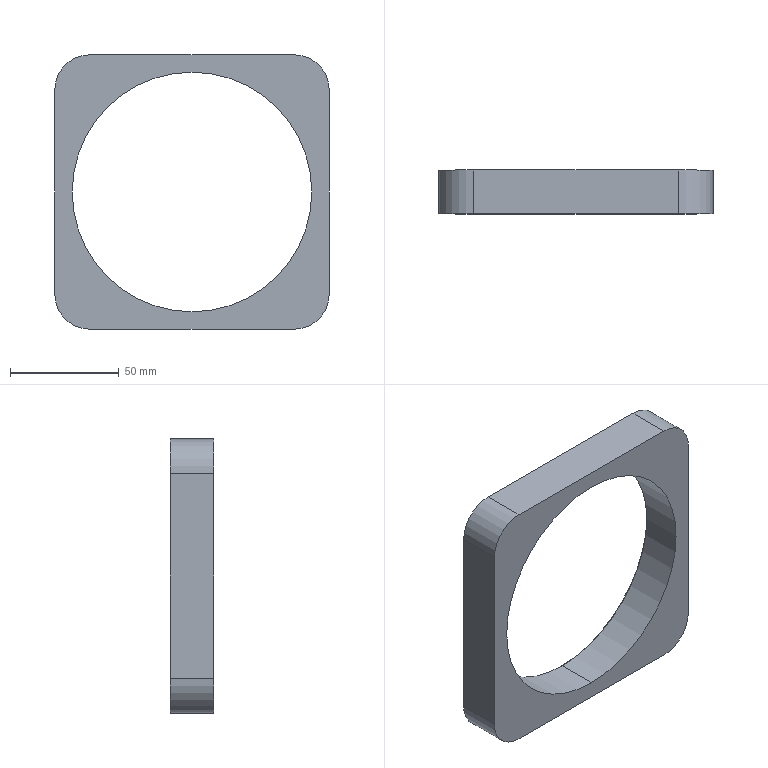Part | SolidWorks | features Chamfer 1, Extrusion 1, HoleWzd 1, ICE 1 | 1 solid | 30 faces | box 126 x 20 x 126 mm | volume 119235 mm3 | cylinder 14 | cone 10 | plane 6 | commonest cylinder face diameters 8.5 x8 32 x4 110 x2
STEP:
#1=CARTESIAN_POINT('',(0.,19.,-55.));
#2=VERTEX_POINT('',#1);
#3=CARTESIAN_POINT('',(0.,19.,55.));
#4=VERTEX_POINT('',#3);
#5=CARTESIAN_POINT('',(0.,19.,0.));
#6=DIRECTION('',(0.,1.,0.));
#7=DIRECTION('',(0.,0.,1.));
#8=AXIS2_PLACEMENT_3D('',#5,#6,#7);
#9=CIRCLE('',#8,55.);
#10=EDGE_CURVE('',#2,#4,#9,.T.);
#11=ORIENTED_EDGE('',*,*,#10,.F.);
#12=CARTESIAN_POINT('',(0.,20.,-56.));
#13=VERTEX_POINT('',#12);
#14=CARTESIAN_POINT('',(0.,19.,-55.));
#15=DIRECTION('',(0.,0.7071,-0.7071));
#16=VECTOR('',#15,1000.);
#17=LINE('',#14,#16);
#18=EDGE_CURVE('',#2,#13,#17,.T.);
#19=ORIENTED_EDGE('',*,*,#18,.T.);
#20=CARTESIAN_POINT('',(0.,20.,56.));
#21=VERTEX_POINT('',#20);
#22=CARTESIAN_POINT('',(0.,20.,0.));
#23=DIRECTION('',(0.,-1.,0.));
#24=DIRECTION('',(0.,0.,1.));
#25=AXIS2_PLACEMENT_3D('',#22,#23,#24);
#26=CIRCLE('',#25,56.);
#27=EDGE_CURVE('',#21,#13,#26,.T.);
#28=ORIENTED_EDGE('',*,*,#27,.F.);
#29=CARTESIAN_POINT('',(0.,19.,55.));
#30=DIRECTION('',(0.,0.7071,0.7071));
#31=VECTOR('',#30,1000.);
#32=LINE('',#29,#31);
#33=EDGE_CURVE('',#4,#21,#32,.T.);
#34=ORIENTED_EDGE('',*,*,#33,.F.);
#35=EDGE_LOOP('',(#11,#19,#28,#34));
#36=FACE_OUTER_BOUND('',#35,.T.);
#37=CARTESIAN_POINT('',(0.,19.,0.));
#38=DIRECTION('',(0.,1.,0.));
#39=DIRECTION('',(0.,0.,1.));
#40=AXIS2_PLACEMENT_3D('',#37,#38,#39);
#41=CONICAL_SURFACE('',#40,55.,0.7854);
#42=ADVANCED_FACE('',(#36),#41,.F.);
#43=CARTESIAN_POINT('',(-47.,4.77,-51.25));
#44=VERTEX_POINT('',#43);
#45=CARTESIAN_POINT('',(-47.,4.77,-42.75));
#46=VERTEX_POINT('',#45);
#47=CARTESIAN_POINT('',(-47.,4.77,-47.));
#48=DIRECTION('',(0.,1.,0.));
#49=DIRECTION('',(0.,0.,1.));
#50=AXIS2_PLACEMENT_3D('',#47,#48,#49);
#51=CIRCLE('',#50,4.25);
#52=EDGE_CURVE('',#44,#46,#51,.T.);
#53=ORIENTED_EDGE('',*,*,#52,.F.);
#54=CARTESIAN_POINT('',(-47.,20.,-51.25));
#55=VERTEX_POINT('',#54);
#56=CARTESIAN_POINT('',(-47.,20.,-51.25));
#57=DIRECTION('',(0.,1.,0.));
#58=VECTOR('',#57,1000.);
#59=LINE('',#56,#58);
#60=EDGE_CURVE('',#44,#55,#59,.T.);
#61=ORIENTED_EDGE('',*,*,#60,.T.);
#62=CARTESIAN_POINT('',(-47.,20.,-42.75));
#63=VERTEX_POINT('',#62);
#64=CARTESIAN_POINT('',(-47.,20.,-47.));
#65=DIRECTION('',(0.,1.,0.));
#66=DIRECTION('',(0.,0.,1.));
#67=AXIS2_PLACEMENT_3D('',#64,#65,#66);
#68=CIRCLE('',#67,4.25);
#69=EDGE_CURVE('',#55,#63,#68,.T.);
#70=ORIENTED_EDGE('',*,*,#69,.T.);
#71=CARTESIAN_POINT('',(-47.,20.,-42.75));
#72=DIRECTION('',(0.,1.,0.));
#73=VECTOR('',#72,1000.);
#74=LINE('',#71,#73);
#75=EDGE_CURVE('',#46,#63,#74,.T.);
#76=ORIENTED_EDGE('',*,*,#75,.F.);
#77=EDGE_LOOP('',(#53,#61,#70,#76));
#78=FACE_OUTER_BOUND('',#77,.T.);
#79=CARTESIAN_POINT('',(-47.,20.,-47.));
#80=DIRECTION('',(0.,1.,0.));
#81=DIRECTION('',(0.,0.,1.));
#82=AXIS2_PLACEMENT_3D('',#79,#80,#81);
#83=CYLINDRICAL_SURFACE('',#82,4.25);
#84=ADVANCED_FACE('',(#78),#83,.F.);
#85=CARTESIAN_POINT('',(-47.,2.216,-47.));
#86=VERTEX_POINT('',#85);
#87=CARTESIAN_POINT('',(-47.,4.77,-42.75));
#88=DIRECTION('',(0.,0.515,0.8572));
#89=VECTOR('',#88,1000.);
#90=LINE('',#87,#89);
#91=EDGE_CURVE('',#86,#46,#90,.T.);
#92=ORIENTED_EDGE('',*,*,#91,.F.);
#93=CARTESIAN_POINT('',(-47.,4.77,-51.25));
#94=DIRECTION('',(0.,0.515,-0.8572));
#95=VECTOR('',#94,1000.);
#96=LINE('',#93,#95);
#97=EDGE_CURVE('',#86,#44,#96,.T.);
#98=ORIENTED_EDGE('',*,*,#97,.T.);
#99=ORIENTED_EDGE('',*,*,#52,.T.);
#100=EDGE_LOOP('',(#92,#98,#99));
#101=FACE_OUTER_BOUND('',#100,.T.);
#102=CARTESIAN_POINT('',(-47.,4.77,-47.));
#103=DIRECTION('',(0.,1.,0.));
#104=DIRECTION('',(0.,0.,1.));
#105=AXIS2_PLACEMENT_3D('',#102,#103,#104);
#106=CONICAL_SURFACE('',#105,4.25,1.03);
#107=ADVANCED_FACE('',(#101),#106,.F.);
#108=CARTESIAN_POINT('',(47.,4.77,-51.25));
#109=VERTEX_POINT('',#108);
#110=CARTESIAN_POINT('',(47.,4.77,-42.75));
#111=VERTEX_POINT('',#110);
#112=CARTESIAN_POINT('',(47.,4.77,-47.));
#113=DIRECTION('',(0.,1.,0.));
#114=DIRECTION('',(0.,0.,1.));
#115=AXIS2_PLACEMENT_3D('',#112,#113,#114);
#116=CIRCLE('',#115,4.25);
#117=EDGE_CURVE('',#109,#111,#116,.T.);
#118=ORIENTED_EDGE('',*,*,#117,.F.);
#119=CARTESIAN_POINT('',(47.,20.,-51.25));
#120=VERTEX_POINT('',#119);
#121=CARTESIAN_POINT('',(47.,20.,-51.25));
#122=DIRECTION('',(0.,1.,0.));
#123=VECTOR('',#122,1000.);
#124=LINE('',#121,#123);
#125=EDGE_CURVE('',#109,#120,#124,.T.);
#126=ORIENTED_EDGE('',*,*,#125,.T.);
#127=CARTESIAN_POINT('',(47.,20.,-42.75));
#128=VERTEX_POINT('',#127);
#129=CARTESIAN_POINT('',(47.,20.,-47.));
#130=DIRECTION('',(0.,1.,0.));
#131=DIRECTION('',(0.,0.,1.));
#132=AXIS2_PLACEMENT_3D('',#129,#130,#131);
#133=CIRCLE('',#132,4.25);
#134=EDGE_CURVE('',#120,#128,#133,.T.);
#135=ORIENTED_EDGE('',*,*,#134,.T.);
#136=CARTESIAN_POINT('',(47.,20.,-42.75));
#137=DIRECTION('',(0.,1.,0.));
#138=VECTOR('',#137,1000.);
#139=LINE('',#136,#138);
#140=EDGE_CURVE('',#111,#128,#139,.T.);
#141=ORIENTED_EDGE('',*,*,#140,.F.);
#142=EDGE_LOOP('',(#118,#126,#135,#141));
#143=FACE_OUTER_BOUND('',#142,.T.);
#144=CARTESIAN_POINT('',(47.,20.,-47.));
#145=DIRECTION('',(0.,1.,0.));
#146=DIRECTION('',(0.,0.,1.));
#147=AXIS2_PLACEMENT_3D('',#144,#145,#146);
#148=CYLINDRICAL_SURFACE('',#147,4.25);
#149=ADVANCED_FACE('',(#143),#148,.F.);
#150=CARTESIAN_POINT('',(47.,2.216,-47.));
#151=VERTEX_POINT('',#150);
#152=CARTESIAN_POINT('',(47.,4.77,-42.75));
#153=DIRECTION('',(0.,0.515,0.8572));
#154=VECTOR('',#153,1000.);
#155=LINE('',#152,#154);
#156=EDGE_CURVE('',#151,#111,#155,.T.);
#157=ORIENTED_EDGE('',*,*,#156,.F.);
#158=CARTESIAN_POINT('',(47.,4.77,-51.25));
#159=DIRECTION('',(0.,0.515,-0.8572));
#160=VECTOR('',#159,1000.);
#161=LINE('',#158,#160);
#162=EDGE_CURVE('',#151,#109,#161,.T.);
#163=ORIENTED_EDGE('',*,*,#162,.T.);
#164=ORIENTED_EDGE('',*,*,#117,.T.);
#165=EDGE_LOOP('',(#157,#163,#164));
#166=FACE_OUTER_BOUND('',#165,.T.);
#167=CARTESIAN_POINT('',(47.,4.77,-47.));
#168=DIRECTION('',(0.,1.,0.));
#169=DIRECTION('',(0.,0.,1.));
#170=AXIS2_PLACEMENT_3D('',#167,#168,#169);
#171=CONICAL_SURFACE('',#170,4.25,1.03);
#172=ADVANCED_FACE('',(#166),#171,.F.);
#173=CARTESIAN_POINT('',(47.,4.77,42.75));
#174=VERTEX_POINT('',#173);
#175=CARTESIAN_POINT('',(47.,4.77,51.25));
#176=VERTEX_POINT('',#175);
#177=CARTESIAN_POINT('',(47.,4.77,47.));
#178=DIRECTION('',(0.,1.,0.));
#179=DIRECTION('',(0.,0.,1.));
#180=AXIS2_PLACEMENT_3D('',#177,#178,#179);
#181=CIRCLE('',#180,4.25);
#182=EDGE_CURVE('',#174,#176,#181,.T.);
#183=ORIENTED_EDGE('',*,*,#182,.F.);
#184=CARTESIAN_POINT('',(47.,20.,42.75));
#185=VERTEX_POINT('',#184);
#186=CARTESIAN_POINT('',(47.,20.,42.75));
#187=DIRECTION('',(0.,1.,0.));
#188=VECTOR('',#187,1000.);
#189=LINE('',#186,#188);
#190=EDGE_CURVE('',#174,#185,#189,.T.);
#191=ORIENTED_EDGE('',*,*,#190,.T.);
#192=CARTESIAN_POINT('',(47.,20.,51.25));
#193=VERTEX_POINT('',#192);
#194=CARTESIAN_POINT('',(47.,20.,47.));
#195=DIRECTION('',(0.,1.,0.));
#196=DIRECTION('',(0.,0.,1.));
#197=AXIS2_PLACEMENT_3D('',#194,#195,#196);
#198=CIRCLE('',#197,4.25);
#199=EDGE_CURVE('',#185,#193,#198,.T.);
#200=ORIENTED_EDGE('',*,*,#199,.T.);
#201=CARTESIAN_POINT('',(47.,20.,51.25));
#202=DIRECTION('',(0.,1.,0.));
#203=VECTOR('',#202,1000.);
#204=LINE('',#201,#203);
#205=EDGE_CURVE('',#176,#193,#204,.T.);
#206=ORIENTED_EDGE('',*,*,#205,.F.);
#207=EDGE_LOOP('',(#183,#191,#200,#206));
#208=FACE_OUTER_BOUND('',#207,.T.);
#209=CARTESIAN_POINT('',(47.,20.,47.));
#210=DIRECTION('',(0.,1.,0.));
#211=DIRECTION('',(0.,0.,1.));
#212=AXIS2_PLACEMENT_3D('',#209,#210,#211);
#213=CYLINDRICAL_SURFACE('',#212,4.25);
#214=ADVANCED_FACE('',(#208),#213,.F.);
#215=CARTESIAN_POINT('',(47.,2.216,47.));
#216=VERTEX_POINT('',#215);
#217=CARTESIAN_POINT('',(47.,4.77,51.25));
#218=DIRECTION('',(0.,0.515,0.8572));
#219=VECTOR('',#218,1000.);
#220=LINE('',#217,#219);
#221=EDGE_CURVE('',#216,#176,#220,.T.);
#222=ORIENTED_EDGE('',*,*,#221,.F.);
#223=CARTESIAN_POINT('',(47.,4.77,42.75));
#224=DIRECTION('',(0.,0.515,-0.8572));
#225=VECTOR('',#224,1000.);
#226=LINE('',#223,#225);
#227=EDGE_CURVE('',#216,#174,#226,.T.);
#228=ORIENTED_EDGE('',*,*,#227,.T.);
#229=ORIENTED_EDGE('',*,*,#182,.T.);
#230=EDGE_LOOP('',(#222,#228,#229));
#231=FACE_OUTER_BOUND('',#230,.T.);
#232=CARTESIAN_POINT('',(47.,4.77,47.));
#233=DIRECTION('',(0.,1.,0.));
#234=DIRECTION('',(0.,0.,1.));
#235=AXIS2_PLACEMENT_3D('',#232,#233,#234);
#236=CONICAL_SURFACE('',#235,4.25,1.03);
#237=ADVANCED_FACE('',(#231),#236,.F.);
#238=CARTESIAN_POINT('',(-47.,4.77,42.75));
#239=VERTEX_POINT('',#238);
#240=CARTESIAN_POINT('',(-47.,4.77,51.25));
#241=VERTEX_POINT('',#240);
#242=CARTESIAN_POINT('',(-47.,4.77,47.));
#243=DIRECTION('',(0.,1.,0.));
#244=DIRECTION('',(0.,0.,1.));
#245=AXIS2_PLACEMENT_3D('',#242,#243,#244);
#246=CIRCLE('',#245,4.25);
#247=EDGE_CURVE('',#239,#241,#246,.T.);
#248=ORIENTED_EDGE('',*,*,#247,.F.);
#249=CARTESIAN_POINT('',(-47.,20.,42.75));
#250=VERTEX_POINT('',#249);
#251=CARTESIAN_POINT('',(-47.,20.,42.75));
#252=DIRECTION('',(0.,1.,0.));
#253=VECTOR('',#252,1000.);
#254=LINE('',#251,#253);
#255=EDGE_CURVE('',#239,#250,#254,.T.);
#256=ORIENTED_EDGE('',*,*,#255,.T.);
#257=CARTESIAN_POINT('',(-47.,20.,51.25));
#258=VERTEX_POINT('',#257);
#259=CARTESIAN_POINT('',(-47.,20.,47.));
#260=DIRECTION('',(0.,1.,0.));
#261=DIRECTION('',(0.,0.,1.));
#262=AXIS2_PLACEMENT_3D('',#259,#260,#261);
#263=CIRCLE('',#262,4.25);
#264=EDGE_CURVE('',#250,#258,#263,.T.);
#265=ORIENTED_EDGE('',*,*,#264,.T.);
#266=CARTESIAN_POINT('',(-47.,20.,51.25));
#267=DIRECTION('',(0.,1.,0.));
#268=VECTOR('',#267,1000.);
#269=LINE('',#266,#268);
#270=EDGE_CURVE('',#241,#258,#269,.T.);
#271=ORIENTED_EDGE('',*,*,#270,.F.);
#272=EDGE_LOOP('',(#248,#256,#265,#271));
#273=FACE_OUTER_BOUND('',#272,.T.);
#274=CARTESIAN_POINT('',(-47.,20.,47.));
#275=DIRECTION('',(0.,1.,0.));
#276=DIRECTION('',(0.,0.,1.));
#277=AXIS2_PLACEMENT_3D('',#274,#275,#276);
#278=CYLINDRICAL_SURFACE('',#277,4.25);
#279=ADVANCED_FACE('',(#273),#278,.F.);
#280=CARTESIAN_POINT('',(-47.,2.216,47.));
#281=VERTEX_POINT('',#280);
#282=CARTESIAN_POINT('',(-47.,4.77,51.25));
#283=DIRECTION('',(0.,0.515,0.8572));
#284=VECTOR('',#283,1000.);
#285=LINE('',#282,#284);
#286=EDGE_CURVE('',#281,#241,#285,.T.);
#287=ORIENTED_EDGE('',*,*,#286,.F.);
#288=CARTESIAN_POINT('',(-47.,4.77,42.75));
#289=DIRECTION('',(0.,0.515,-0.8572));
#290=VECTOR('',#289,1000.);
#291=LINE('',#288,#290);
#292=EDGE_CURVE('',#281,#239,#291,.T.);
#293=ORIENTED_EDGE('',*,*,#292,.T.);
#294=ORIENTED_EDGE('',*,*,#247,.T.);
#295=EDGE_LOOP('',(#287,#293,#294));
#296=FACE_OUTER_BOUND('',#295,.T.);
#297=CARTESIAN_POINT('',(-47.,4.77,47.));
#298=DIRECTION('',(0.,1.,0.));
#299=DIRECTION('',(0.,0.,1.));
#300=AXIS2_PLACEMENT_3D('',#297,#298,#299);
#301=CONICAL_SURFACE('',#300,4.25,1.03);
#302=ADVANCED_FACE('',(#296),#301,.F.);
#303=ORIENTED_EDGE('',*,*,#10,.T.);
#304=CARTESIAN_POINT('',(0.,0.,55.));
#305=VERTEX_POINT('',#304);
#306=CARTESIAN_POINT('',(0.,20.,55.));
#307=DIRECTION('',(0.,-1.,0.));
#308=VECTOR('',#307,1000.);
#309=LINE('',#306,#308);
#310=EDGE_CURVE('',#4,#305,#309,.T.);
#311=ORIENTED_EDGE('',*,*,#310,.T.);
#312=CARTESIAN_POINT('',(0.,0.,-55.));
#313=VERTEX_POINT('',#312);
#314=CARTESIAN_POINT('',(0.,0.,0.));
#315=DIRECTION('',(0.,1.,0.));
#316=DIRECTION('',(0.,0.,1.));
#317=AXIS2_PLACEMENT_3D('',#314,#315,#316);
#318=CIRCLE('',#317,55.);
#319=EDGE_CURVE('',#313,#305,#318,.T.);
#320=ORIENTED_EDGE('',*,*,#319,.F.);
#321=CARTESIAN_POINT('',(0.,20.,-55.));
#322=DIRECTION('',(0.,-1.,0.));
#323=VECTOR('',#322,1000.);
#324=LINE('',#321,#323);
#325=EDGE_CURVE('',#2,#313,#324,.T.);
#326=ORIENTED_EDGE('',*,*,#325,.F.);
#327=EDGE_LOOP('',(#303,#311,#320,#326));
#328=FACE_OUTER_BOUND('',#327,.T.);
#329=CARTESIAN_POINT('',(0.,20.,0.));
#330=DIRECTION('',(0.,-1.,0.));
#331=DIRECTION('',(0.,0.,-1.));
#332=AXIS2_PLACEMENT_3D('',#329,#330,#331);
#333=CYLINDRICAL_SURFACE('',#332,55.);
#334=ADVANCED_FACE('',(#328),#333,.F.);
#335=ORIENTED_EDGE('',*,*,#27,.T.);
#336=CARTESIAN_POINT('',(0.,20.,0.));
#337=DIRECTION('',(0.,-1.,0.));
#338=DIRECTION('',(0.,0.,1.));
#339=AXIS2_PLACEMENT_3D('',#336,#337,#338);
#340=CIRCLE('',#339,56.);
#341=EDGE_CURVE('',#13,#21,#340,.T.);
#342=ORIENTED_EDGE('',*,*,#341,.T.);
#343=EDGE_LOOP('',(#335,#342));
#344=FACE_BOUND('',#343,.T.);
#345=CARTESIAN_POINT('',(-47.,20.,-47.));
#346=DIRECTION('',(0.,1.,0.));
#347=DIRECTION('',(0.,0.,1.));
#348=AXIS2_PLACEMENT_3D('',#345,#346,#347);
#349=CIRCLE('',#348,4.25);
#350=EDGE_CURVE('',#63,#55,#349,.T.);
#351=ORIENTED_EDGE('',*,*,#350,.F.);
#352=ORIENTED_EDGE('',*,*,#69,.F.);
#353=EDGE_LOOP('',(#351,#352));
#354=FACE_BOUND('',#353,.T.);
#355=CARTESIAN_POINT('',(47.,20.,-47.));
#356=DIRECTION('',(0.,1.,0.));
#357=DIRECTION('',(0.,0.,1.));
#358=AXIS2_PLACEMENT_3D('',#355,#356,#357);
#359=CIRCLE('',#358,4.25);
#360=EDGE_CURVE('',#128,#120,#359,.T.);
#361=ORIENTED_EDGE('',*,*,#360,.F.);
#362=ORIENTED_EDGE('',*,*,#134,.F.);
#363=EDGE_LOOP('',(#361,#362));
#364=FACE_BOUND('',#363,.T.);
#365=CARTESIAN_POINT('',(47.,20.,47.));
#366=DIRECTION('',(0.,1.,0.));
#367=DIRECTION('',(0.,0.,1.));
#368=AXIS2_PLACEMENT_3D('',#365,#366,#367);
#369=CIRCLE('',#368,4.25);
#370=EDGE_CURVE('',#193,#185,#369,.T.);
#371=ORIENTED_EDGE('',*,*,#370,.F.);
#372=ORIENTED_EDGE('',*,*,#199,.F.);
#373=EDGE_LOOP('',(#371,#372));
#374=FACE_BOUND('',#373,.T.);
#375=CARTESIAN_POINT('',(-47.,20.,47.));
#376=DIRECTION('',(0.,1.,0.));
#377=DIRECTION('',(0.,0.,1.));
#378=AXIS2_PLACEMENT_3D('',#375,#376,#377);
#379=CIRCLE('',#378,4.25);
#380=EDGE_CURVE('',#258,#250,#379,.T.);
#381=ORIENTED_EDGE('',*,*,#380,.F.);
#382=ORIENTED_EDGE('',*,*,#264,.F.);
#383=EDGE_LOOP('',(#381,#382));
#384=FACE_BOUND('',#383,.T.);
#385=CARTESIAN_POINT('',(-63.,20.,47.));
#386=VERTEX_POINT('',#385);
#387=CARTESIAN_POINT('',(-47.,20.,63.));
#388=VERTEX_POINT('',#387);
#389=CARTESIAN_POINT('',(-47.,20.,47.));
#390=DIRECTION('',(0.,1.,0.));
#391=DIRECTION('',(0.,0.,1.));
#392=AXIS2_PLACEMENT_3D('',#389,#390,#391);
#393=CIRCLE('',#392,16.);
#394=EDGE_CURVE('',#386,#388,#393,.T.);
#395=ORIENTED_EDGE('',*,*,#394,.T.);
#396=CARTESIAN_POINT('',(47.,20.,63.));
#397=VERTEX_POINT('',#396);
#398=CARTESIAN_POINT('',(-47.,20.,63.));
#399=DIRECTION('',(1.,0.,0.));
#400=VECTOR('',#399,1000.);
#401=LINE('',#398,#400);
#402=EDGE_CURVE('',#388,#397,#401,.T.);
#403=ORIENTED_EDGE('',*,*,#402,.T.);
#404=CARTESIAN_POINT('',(63.,20.,47.));
#405=VERTEX_POINT('',#404);
#406=CARTESIAN_POINT('',(47.,20.,47.));
#407=DIRECTION('',(0.,1.,0.));
#408=DIRECTION('',(0.,0.,1.));
#409=AXIS2_PLACEMENT_3D('',#406,#407,#408);
#410=CIRCLE('',#409,16.);
#411=EDGE_CURVE('',#397,#405,#410,.T.);
#412=ORIENTED_EDGE('',*,*,#411,.T.);
#413=CARTESIAN_POINT('',(63.,20.,-47.));
#414=VERTEX_POINT('',#413);
#415=CARTESIAN_POINT('',(63.,20.,-47.));
#416=DIRECTION('',(0.,0.,-1.));
#417=VECTOR('',#416,1000.);
#418=LINE('',#415,#417);
#419=EDGE_CURVE('',#405,#414,#418,.T.);
#420=ORIENTED_EDGE('',*,*,#419,.T.);
#421=CARTESIAN_POINT('',(47.,20.,-63.));
#422=VERTEX_POINT('',#421);
#423=CARTESIAN_POINT('',(47.,20.,-47.));
#424=DIRECTION('',(0.,1.,0.));
#425=DIRECTION('',(0.,0.,-1.));
#426=AXIS2_PLACEMENT_3D('',#423,#424,#425);
#427=CIRCLE('',#426,16.);
#428=EDGE_CURVE('',#414,#422,#427,.T.);
#429=ORIENTED_EDGE('',*,*,#428,.T.);
#430=CARTESIAN_POINT('',(-47.,20.,-63.));
#431=VERTEX_POINT('',#430);
#432=CARTESIAN_POINT('',(-47.,20.,-63.));
#433=DIRECTION('',(-1.,0.,0.));
#434=VECTOR('',#433,1000.);
#435=LINE('',#432,#434);
#436=EDGE_CURVE('',#422,#431,#435,.T.);
#437=ORIENTED_EDGE('',*,*,#436,.T.);
#438=CARTESIAN_POINT('',(-63.,20.,-47.));
#439=VERTEX_POINT('',#438);
#440=CARTESIAN_POINT('',(-47.,20.,-47.));
#441=DIRECTION('',(0.,1.,0.));
#442=DIRECTION('',(0.,0.,1.));
#443=AXIS2_PLACEMENT_3D('',#440,#441,#442);
#444=CIRCLE('',#443,16.);
#445=EDGE_CURVE('',#431,#439,#444,.T.);
#446=ORIENTED_EDGE('',*,*,#445,.T.);
#447=CARTESIAN_POINT('',(-63.,20.,-47.));
#448=DIRECTION('',(0.,0.,1.));
#449=VECTOR('',#448,1000.);
#450=LINE('',#447,#449);
#451=EDGE_CURVE('',#439,#386,#450,.T.);
#452=ORIENTED_EDGE('',*,*,#451,.T.);
#453=EDGE_LOOP('',(#395,#403,#412,#420,#429,#437,#446,#452));
#454=FACE_OUTER_BOUND('',#453,.T.);
#455=CARTESIAN_POINT('',(-47.,20.,47.));
#456=DIRECTION('',(0.,1.,0.));
#457=DIRECTION('',(0.,0.,1.));
#458=AXIS2_PLACEMENT_3D('',#455,#456,#457);
#459=PLANE('',#458);
#460=ADVANCED_FACE('',(#344,#354,#364,#374,#384,#454),#459,.T.);
#461=CARTESIAN_POINT('',(-63.,0.,47.));
#462=VERTEX_POINT('',#461);
#463=CARTESIAN_POINT('',(-47.,0.,63.));
#464=VERTEX_POINT('',#463);
#465=CARTESIAN_POINT('',(-47.,0.,47.));
#466=DIRECTION('',(0.,1.,0.));
#467=DIRECTION('',(0.,0.,1.));
#468=AXIS2_PLACEMENT_3D('',#465,#466,#467);
#469=CIRCLE('',#468,16.);
#470=EDGE_CURVE('',#462,#464,#469,.T.);
#471=ORIENTED_EDGE('',*,*,#470,.F.);
#472=CARTESIAN_POINT('',(-63.,0.,-47.));
#473=VERTEX_POINT('',#472);
#474=CARTESIAN_POINT('',(-63.,0.,-47.));
#475=DIRECTION('',(0.,0.,1.));
#476=VECTOR('',#475,1000.);
#477=LINE('',#474,#476);
#478=EDGE_CURVE('',#473,#462,#477,.T.);
#479=ORIENTED_EDGE('',*,*,#478,.F.);
#480=CARTESIAN_POINT('',(-47.,0.,-63.));
#481=VERTEX_POINT('',#480);
#482=CARTESIAN_POINT('',(-47.,0.,-47.));
#483=DIRECTION('',(0.,1.,0.));
#484=DIRECTION('',(0.,0.,1.));
#485=AXIS2_PLACEMENT_3D('',#482,#483,#484);
#486=CIRCLE('',#485,16.);
#487=EDGE_CURVE('',#481,#473,#486,.T.);
#488=ORIENTED_EDGE('',*,*,#487,.F.);
#489=CARTESIAN_POINT('',(47.,0.,-63.));
#490=VERTEX_POINT('',#489);
#491=CARTESIAN_POINT('',(-47.,0.,-63.));
#492=DIRECTION('',(-1.,0.,0.));
#493=VECTOR('',#492,1000.);
#494=LINE('',#491,#493);
#495=EDGE_CURVE('',#490,#481,#494,.T.);
#496=ORIENTED_EDGE('',*,*,#495,.F.);
#497=CARTESIAN_POINT('',(63.,0.,-47.));
#498=VERTEX_POINT('',#497);
#499=CARTESIAN_POINT('',(47.,0.,-47.));
#500=DIRECTION('',(0.,1.,0.));
#501=DIRECTION('',(0.,0.,-1.));
#502=AXIS2_PLACEMENT_3D('',#499,#500,#501);
#503=CIRCLE('',#502,16.);
#504=EDGE_CURVE('',#498,#490,#503,.T.);
#505=ORIENTED_EDGE('',*,*,#504,.F.);
#506=CARTESIAN_POINT('',(63.,0.,47.));
#507=VERTEX_POINT('',#506);
#508=CARTESIAN_POINT('',(63.,0.,-47.));
#509=DIRECTION('',(0.,0.,-1.));
#510=VECTOR('',#509,1000.);
#511=LINE('',#508,#510);
#512=EDGE_CURVE('',#507,#498,#511,.T.);
#513=ORIENTED_EDGE('',*,*,#512,.F.);
#514=CARTESIAN_POINT('',(47.,0.,63.));
#515=VERTEX_POINT('',#514);
#516=CARTESIAN_POINT('',(47.,0.,47.));
#517=DIRECTION('',(0.,1.,0.));
#518=DIRECTION('',(0.,0.,1.));
#519=AXIS2_PLACEMENT_3D('',#516,#517,#518);
#520=CIRCLE('',#519,16.);
#521=EDGE_CURVE('',#515,#507,#520,.T.);
#522=ORIENTED_EDGE('',*,*,#521,.F.);
#523=CARTESIAN_POINT('',(-47.,0.,63.));
#524=DIRECTION('',(1.,0.,0.));
#525=VECTOR('',#524,1000.);
#526=LINE('',#523,#525);
#527=EDGE_CURVE('',#464,#515,#526,.T.);
#528=ORIENTED_EDGE('',*,*,#527,.F.);
#529=EDGE_LOOP('',(#471,#479,#488,#496,#505,#513,#522,#528));
#530=FACE_OUTER_BOUND('',#529,.T.);
#531=ORIENTED_EDGE('',*,*,#319,.T.);
#532=CARTESIAN_POINT('',(0.,0.,0.));
#533=DIRECTION('',(0.,1.,0.));
#534=DIRECTION('',(0.,0.,1.));
#535=AXIS2_PLACEMENT_3D('',#532,#533,#534);
#536=CIRCLE('',#535,55.);
#537=EDGE_CURVE('',#305,#313,#536,.T.);
#538=ORIENTED_EDGE('',*,*,#537,.T.);
#539=EDGE_LOOP('',(#531,#538));
#540=FACE_BOUND('',#539,.T.);
#541=CARTESIAN_POINT('',(-47.,0.,47.));
#542=DIRECTION('',(0.,1.,0.));
#543=DIRECTION('',(0.,0.,1.));
#544=AXIS2_PLACEMENT_3D('',#541,#542,#543);
#545=PLANE('',#544);
#546=ADVANCED_FACE('',(#530,#540),#545,.F.);
#547=ORIENTED_EDGE('',*,*,#470,.T.);
#548=CARTESIAN_POINT('',(-47.,20.,63.));
#549=DIRECTION('',(0.,-1.,0.));
#550=VECTOR('',#549,1000.);
#551=LINE('',#548,#550);
#552=EDGE_CURVE('',#388,#464,#551,.T.);
#553=ORIENTED_EDGE('',*,*,#552,.F.);
#554=ORIENTED_EDGE('',*,*,#394,.F.);
#555=CARTESIAN_POINT('',(-63.,20.,47.));
#556=DIRECTION('',(0.,-1.,0.));
#557=VECTOR('',#556,1000.);
#558=LINE('',#555,#557);
#559=EDGE_CURVE('',#386,#462,#558,.T.);
#560=ORIENTED_EDGE('',*,*,#559,.T.);
#561=EDGE_LOOP('',(#547,#553,#554,#560));
#562=FACE_OUTER_BOUND('',#561,.T.);
#563=CARTESIAN_POINT('',(-47.,20.,47.));
#564=DIRECTION('',(0.,-1.,0.));
#565=DIRECTION('',(0.,0.,-1.));
#566=AXIS2_PLACEMENT_3D('',#563,#564,#565);
#567=CYLINDRICAL_SURFACE('',#566,16.);
#568=ADVANCED_FACE('',(#562),#567,.T.);
#569=ORIENTED_EDGE('',*,*,#527,.T.);
#570=CARTESIAN_POINT('',(47.,20.,63.));
#571=DIRECTION('',(0.,-1.,0.));
#572=VECTOR('',#571,1000.);
#573=LINE('',#570,#572);
#574=EDGE_CURVE('',#397,#515,#573,.T.);
#575=ORIENTED_EDGE('',*,*,#574,.F.);
#576=ORIENTED_EDGE('',*,*,#402,.F.);
#577=ORIENTED_EDGE('',*,*,#552,.T.);
#578=EDGE_LOOP('',(#569,#575,#576,#577));
#579=FACE_OUTER_BOUND('',#578,.T.);
#580=CARTESIAN_POINT('',(-47.,20.,63.));
#581=DIRECTION('',(0.,0.,-1.));
#582=DIRECTION('',(-1.,0.,0.));
#583=AXIS2_PLACEMENT_3D('',#580,#581,#582);
#584=PLANE('',#583);
#585=ADVANCED_FACE('',(#579),#584,.F.);
#586=ORIENTED_EDGE('',*,*,#521,.T.);
#587=CARTESIAN_POINT('',(63.,20.,47.));
#588=DIRECTION('',(0.,-1.,0.));
#589=VECTOR('',#588,1000.);
#590=LINE('',#587,#589);
#591=EDGE_CURVE('',#405,#507,#590,.T.);
#592=ORIENTED_EDGE('',*,*,#591,.F.);
#593=ORIENTED_EDGE('',*,*,#411,.F.);
#594=ORIENTED_EDGE('',*,*,#574,.T.);
#595=EDGE_LOOP('',(#586,#592,#593,#594));
#596=FACE_OUTER_BOUND('',#595,.T.);
#597=CARTESIAN_POINT('',(47.,20.,47.));
#598=DIRECTION('',(0.,-1.,0.));
#599=DIRECTION('',(0.,0.,-1.));
#600=AXIS2_PLACEMENT_3D('',#597,#598,#599);
#601=CYLINDRICAL_SURFACE('',#600,16.);
#602=ADVANCED_FACE('',(#596),#601,.T.);
#603=ORIENTED_EDGE('',*,*,#512,.T.);
#604=CARTESIAN_POINT('',(63.,20.,-47.));
#605=DIRECTION('',(0.,-1.,0.));
#606=VECTOR('',#605,1000.);
#607=LINE('',#604,#606);
#608=EDGE_CURVE('',#414,#498,#607,.T.);
#609=ORIENTED_EDGE('',*,*,#608,.F.);
#610=ORIENTED_EDGE('',*,*,#419,.F.);
#611=ORIENTED_EDGE('',*,*,#591,.T.);
#612=EDGE_LOOP('',(#603,#609,#610,#611));
#613=FACE_OUTER_BOUND('',#612,.T.);
#614=CARTESIAN_POINT('',(63.,20.,-47.));
#615=DIRECTION('',(-1.,0.,0.));
#616=DIRECTION('',(0.,0.,1.));
#617=AXIS2_PLACEMENT_3D('',#614,#615,#616);
#618=PLANE('',#617);
#619=ADVANCED_FACE('',(#613),#618,.F.);
#620=ORIENTED_EDGE('',*,*,#504,.T.);
#621=CARTESIAN_POINT('',(47.,20.,-63.));
#622=DIRECTION('',(0.,-1.,0.));
#623=VECTOR('',#622,1000.);
#624=LINE('',#621,#623);
#625=EDGE_CURVE('',#422,#490,#624,.T.);
#626=ORIENTED_EDGE('',*,*,#625,.F.);
#627=ORIENTED_EDGE('',*,*,#428,.F.);
#628=ORIENTED_EDGE('',*,*,#608,.T.);
#629=EDGE_LOOP('',(#620,#626,#627,#628));
#630=FACE_OUTER_BOUND('',#629,.T.);
#631=CARTESIAN_POINT('',(47.,20.,-47.));
#632=DIRECTION('',(0.,-1.,0.));
#633=DIRECTION('',(0.,0.,-1.));
#634=AXIS2_PLACEMENT_3D('',#631,#632,#633);
#635=CYLINDRICAL_SURFACE('',#634,16.);
#636=ADVANCED_FACE('',(#630),#635,.T.);
#637=ORIENTED_EDGE('',*,*,#495,.T.);
#638=CARTESIAN_POINT('',(-47.,20.,-63.));
#639=DIRECTION('',(0.,-1.,0.));
#640=VECTOR('',#639,1000.);
#641=LINE('',#638,#640);
#642=EDGE_CURVE('',#431,#481,#641,.T.);
#643=ORIENTED_EDGE('',*,*,#642,.F.);
#644=ORIENTED_EDGE('',*,*,#436,.F.);
#645=ORIENTED_EDGE('',*,*,#625,.T.);
#646=EDGE_LOOP('',(#637,#643,#644,#645));
#647=FACE_OUTER_BOUND('',#646,.T.);
#648=CARTESIAN_POINT('',(-47.,20.,-63.));
#649=DIRECTION('',(0.,0.,1.));
#650=DIRECTION('',(1.,0.,0.));
#651=AXIS2_PLACEMENT_3D('',#648,#649,#650);
#652=PLANE('',#651);
#653=ADVANCED_FACE('',(#647),#652,.F.);
#654=ORIENTED_EDGE('',*,*,#487,.T.);
#655=CARTESIAN_POINT('',(-63.,20.,-47.));
#656=DIRECTION('',(0.,-1.,0.));
#657=VECTOR('',#656,1000.);
#658=LINE('',#655,#657);
#659=EDGE_CURVE('',#439,#473,#658,.T.);
#660=ORIENTED_EDGE('',*,*,#659,.F.);
#661=ORIENTED_EDGE('',*,*,#445,.F.);
#662=ORIENTED_EDGE('',*,*,#642,.T.);
#663=EDGE_LOOP('',(#654,#660,#661,#662));
#664=FACE_OUTER_BOUND('',#663,.T.);
#665=CARTESIAN_POINT('',(-47.,20.,-47.));
#666=DIRECTION('',(0.,-1.,0.));
#667=DIRECTION('',(0.,0.,-1.));
#668=AXIS2_PLACEMENT_3D('',#665,#666,#667);
#669=CYLINDRICAL_SURFACE('',#668,16.);
#670=ADVANCED_FACE('',(#664),#669,.T.);
#671=ORIENTED_EDGE('',*,*,#478,.T.);
#672=ORIENTED_EDGE('',*,*,#559,.F.);
#673=ORIENTED_EDGE('',*,*,#451,.F.);
#674=ORIENTED_EDGE('',*,*,#659,.T.);
#675=EDGE_LOOP('',(#671,#672,#673,#674));
#676=FACE_OUTER_BOUND('',#675,.T.);
#677=CARTESIAN_POINT('',(-63.,20.,-47.));
#678=DIRECTION('',(1.,0.,0.));
#679=DIRECTION('',(0.,0.,-1.));
#680=AXIS2_PLACEMENT_3D('',#677,#678,#679);
#681=PLANE('',#680);
#682=ADVANCED_FACE('',(#676),#681,.F.);
#683=ORIENTED_EDGE('',*,*,#310,.F.);
#684=CARTESIAN_POINT('',(0.,19.,0.));
#685=DIRECTION('',(0.,1.,0.));
#686=DIRECTION('',(0.,0.,1.));
#687=AXIS2_PLACEMENT_3D('',#684,#685,#686);
#688=CIRCLE('',#687,55.);
#689=EDGE_CURVE('',#4,#2,#688,.T.);
#690=ORIENTED_EDGE('',*,*,#689,.T.);
#691=ORIENTED_EDGE('',*,*,#325,.T.);
#692=ORIENTED_EDGE('',*,*,#537,.F.);
#693=EDGE_LOOP('',(#683,#690,#691,#692));
#694=FACE_OUTER_BOUND('',#693,.T.);
#695=CARTESIAN_POINT('',(0.,20.,0.));
#696=DIRECTION('',(0.,-1.,0.));
#697=DIRECTION('',(0.,0.,-1.));
#698=AXIS2_PLACEMENT_3D('',#695,#696,#697);
#699=CYLINDRICAL_SURFACE('',#698,55.);
#700=ADVANCED_FACE('',(#694),#699,.F.);
#701=ORIENTED_EDGE('',*,*,#292,.F.);
#702=ORIENTED_EDGE('',*,*,#286,.T.);
#703=CARTESIAN_POINT('',(-47.,4.77,47.));
#704=DIRECTION('',(0.,1.,0.));
#705=DIRECTION('',(0.,0.,1.));
#706=AXIS2_PLACEMENT_3D('',#703,#704,#705);
#707=CIRCLE('',#706,4.25);
#708=EDGE_CURVE('',#241,#239,#707,.T.);
#709=ORIENTED_EDGE('',*,*,#708,.T.);
#710=EDGE_LOOP('',(#701,#702,#709));
#711=FACE_OUTER_BOUND('',#710,.T.);
#712=CARTESIAN_POINT('',(-47.,4.77,47.));
#713=DIRECTION('',(0.,1.,0.));
#714=DIRECTION('',(0.,0.,1.));
#715=AXIS2_PLACEMENT_3D('',#712,#713,#714);
#716=CONICAL_SURFACE('',#715,4.25,1.03);
#717=ADVANCED_FACE('',(#711),#716,.F.);
#718=ORIENTED_EDGE('',*,*,#255,.F.);
#719=ORIENTED_EDGE('',*,*,#708,.F.);
#720=ORIENTED_EDGE('',*,*,#270,.T.);
#721=ORIENTED_EDGE('',*,*,#380,.T.);
#722=EDGE_LOOP('',(#718,#719,#720,#721));
#723=FACE_OUTER_BOUND('',#722,.T.);
#724=CARTESIAN_POINT('',(-47.,20.,47.));
#725=DIRECTION('',(0.,1.,0.));
#726=DIRECTION('',(0.,0.,1.));
#727=AXIS2_PLACEMENT_3D('',#724,#725,#726);
#728=CYLINDRICAL_SURFACE('',#727,4.25);
#729=ADVANCED_FACE('',(#723),#728,.F.);
#730=ORIENTED_EDGE('',*,*,#227,.F.);
#731=ORIENTED_EDGE('',*,*,#221,.T.);
#732=CARTESIAN_POINT('',(47.,4.77,47.));
#733=DIRECTION('',(0.,1.,0.));
#734=DIRECTION('',(0.,0.,1.));
#735=AXIS2_PLACEMENT_3D('',#732,#733,#734);
#736=CIRCLE('',#735,4.25);
#737=EDGE_CURVE('',#176,#174,#736,.T.);
#738=ORIENTED_EDGE('',*,*,#737,.T.);
#739=EDGE_LOOP('',(#730,#731,#738));
#740=FACE_OUTER_BOUND('',#739,.T.);
#741=CARTESIAN_POINT('',(47.,4.77,47.));
#742=DIRECTION('',(0.,1.,0.));
#743=DIRECTION('',(0.,0.,1.));
#744=AXIS2_PLACEMENT_3D('',#741,#742,#743);
#745=CONICAL_SURFACE('',#744,4.25,1.03);
#746=ADVANCED_FACE('',(#740),#745,.F.);
#747=ORIENTED_EDGE('',*,*,#190,.F.);
#748=ORIENTED_EDGE('',*,*,#737,.F.);
#749=ORIENTED_EDGE('',*,*,#205,.T.);
#750=ORIENTED_EDGE('',*,*,#370,.T.);
#751=EDGE_LOOP('',(#747,#748,#749,#750));
#752=FACE_OUTER_BOUND('',#751,.T.);
#753=CARTESIAN_POINT('',(47.,20.,47.));
#754=DIRECTION('',(0.,1.,0.));
#755=DIRECTION('',(0.,0.,1.));
#756=AXIS2_PLACEMENT_3D('',#753,#754,#755);
#757=CYLINDRICAL_SURFACE('',#756,4.25);
#758=ADVANCED_FACE('',(#752),#757,.F.);
#759=ORIENTED_EDGE('',*,*,#162,.F.);
#760=ORIENTED_EDGE('',*,*,#156,.T.);
#761=CARTESIAN_POINT('',(47.,4.77,-47.));
#762=DIRECTION('',(0.,1.,0.));
#763=DIRECTION('',(0.,0.,1.));
#764=AXIS2_PLACEMENT_3D('',#761,#762,#763);
#765=CIRCLE('',#764,4.25);
#766=EDGE_CURVE('',#111,#109,#765,.T.);
#767=ORIENTED_EDGE('',*,*,#766,.T.);
#768=EDGE_LOOP('',(#759,#760,#767));
#769=FACE_OUTER_BOUND('',#768,.T.);
#770=CARTESIAN_POINT('',(47.,4.77,-47.));
#771=DIRECTION('',(0.,1.,0.));
#772=DIRECTION('',(0.,0.,1.));
#773=AXIS2_PLACEMENT_3D('',#770,#771,#772);
#774=CONICAL_SURFACE('',#773,4.25,1.03);
#775=ADVANCED_FACE('',(#769),#774,.F.);
#776=ORIENTED_EDGE('',*,*,#125,.F.);
#777=ORIENTED_EDGE('',*,*,#766,.F.);
#778=ORIENTED_EDGE('',*,*,#140,.T.);
#779=ORIENTED_EDGE('',*,*,#360,.T.);
#780=EDGE_LOOP('',(#776,#777,#778,#779));
#781=FACE_OUTER_BOUND('',#780,.T.);
#782=CARTESIAN_POINT('',(47.,20.,-47.));
#783=DIRECTION('',(0.,1.,0.));
#784=DIRECTION('',(0.,0.,1.));
#785=AXIS2_PLACEMENT_3D('',#782,#783,#784);
#786=CYLINDRICAL_SURFACE('',#785,4.25);
#787=ADVANCED_FACE('',(#781),#786,.F.);
#788=ORIENTED_EDGE('',*,*,#97,.F.);
#789=ORIENTED_EDGE('',*,*,#91,.T.);
#790=CARTESIAN_POINT('',(-47.,4.77,-47.));
#791=DIRECTION('',(0.,1.,0.));
#792=DIRECTION('',(0.,0.,1.));
#793=AXIS2_PLACEMENT_3D('',#790,#791,#792);
#794=CIRCLE('',#793,4.25);
#795=EDGE_CURVE('',#46,#44,#794,.T.);
#796=ORIENTED_EDGE('',*,*,#795,.T.);
#797=EDGE_LOOP('',(#788,#789,#796));
#798=FACE_OUTER_BOUND('',#797,.T.);
#799=CARTESIAN_POINT('',(-47.,4.77,-47.));
#800=DIRECTION('',(0.,1.,0.));
#801=DIRECTION('',(0.,0.,1.));
#802=AXIS2_PLACEMENT_3D('',#799,#800,#801);
#803=CONICAL_SURFACE('',#802,4.25,1.03);
#804=ADVANCED_FACE('',(#798),#803,.F.);
#805=ORIENTED_EDGE('',*,*,#60,.F.);
#806=ORIENTED_EDGE('',*,*,#795,.F.);
#807=ORIENTED_EDGE('',*,*,#75,.T.);
#808=ORIENTED_EDGE('',*,*,#350,.T.);
#809=EDGE_LOOP('',(#805,#806,#807,#808));
#810=FACE_OUTER_BOUND('',#809,.T.);
#811=CARTESIAN_POINT('',(-47.,20.,-47.));
#812=DIRECTION('',(0.,1.,0.));
#813=DIRECTION('',(0.,0.,1.));
#814=AXIS2_PLACEMENT_3D('',#811,#812,#813);
#815=CYLINDRICAL_SURFACE('',#814,4.25);
#816=ADVANCED_FACE('',(#810),#815,.F.);
#817=ORIENTED_EDGE('',*,*,#18,.F.);
#818=ORIENTED_EDGE('',*,*,#689,.F.);
#819=ORIENTED_EDGE('',*,*,#33,.T.);
#820=ORIENTED_EDGE('',*,*,#341,.F.);
#821=EDGE_LOOP('',(#817,#818,#819,#820));
#822=FACE_OUTER_BOUND('',#821,.T.);
#823=CARTESIAN_POINT('',(0.,19.,0.));
#824=DIRECTION('',(0.,1.,0.));
#825=DIRECTION('',(0.,0.,1.));
#826=AXIS2_PLACEMENT_3D('',#823,#824,#825);
#827=CONICAL_SURFACE('',#826,55.,0.7854);
#828=ADVANCED_FACE('',(#822),#827,.F.);
#829=CLOSED_SHELL('',(#42,#84,#107,#149,#172,#214,#237,#279,#302,#334,#460,#546,#568,#585,#602,#619,#636,#653,#670,#682,#700,#717,#729,#746,#758,#775,#787,#804,#816,#828));
#830=MANIFOLD_SOLID_BREP('',#829);
#831=CARTESIAN_POINT('',(0.,0.,0.));
#832=DIRECTION('',(0.,0.,1.));
#833=DIRECTION('',(1.,0.,0.));
#834=AXIS2_PLACEMENT_3D('',#831,#832,#833);
#835=(LENGTH_UNIT()NAMED_UNIT(*)SI_UNIT(.MILLI.,.METRE.));
#836=UNCERTAINTY_MEASURE_WITH_UNIT(LENGTH_MEASURE(0.00001),#835,'','');
#837=(NAMED_UNIT(*)PLANE_ANGLE_UNIT()SI_UNIT($,.RADIAN.));
#838=(NAMED_UNIT(*)SI_UNIT($,.STERADIAN.)SOLID_ANGLE_UNIT());
#839=(GEOMETRIC_REPRESENTATION_CONTEXT(3)GLOBAL_UNCERTAINTY_ASSIGNED_CONTEXT((#836))GLOBAL_UNIT_ASSIGNED_CONTEXT((#835,#837,#838))REPRESENTATION_CONTEXT('',''));
#840=ADVANCED_BREP_SHAPE_REPRESENTATION('',(#830,#834),#839);